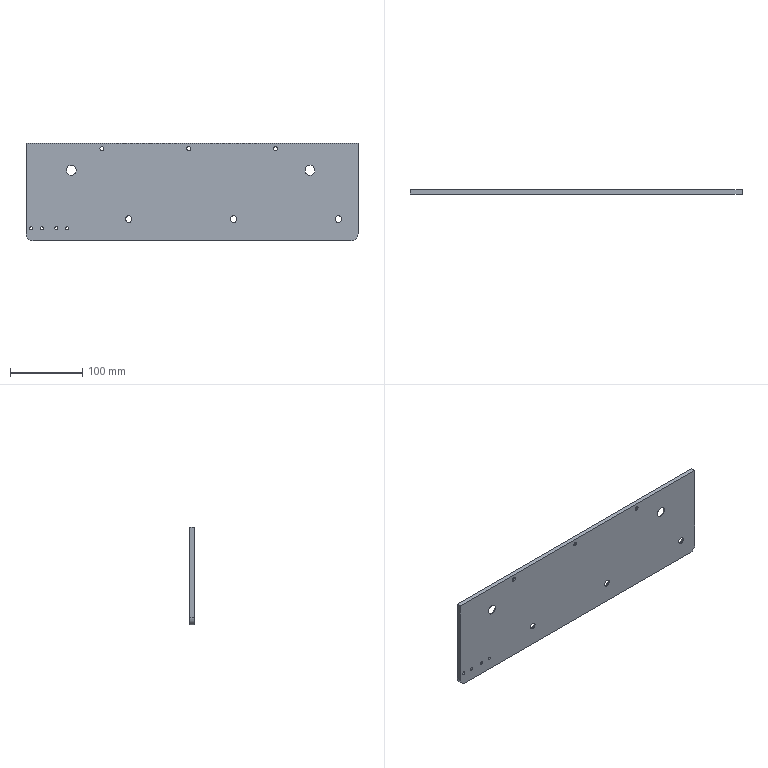Part | STEP file | 1 solid | 48 faces | box 459 x 6 x 135 mm | volume 364434 mm3 | cylinder 26 | cone 16 | plane 6 | commonest cylinder face diameters 4.2 x8 5.5 x6 9 x6 13.5 x4 20 x2